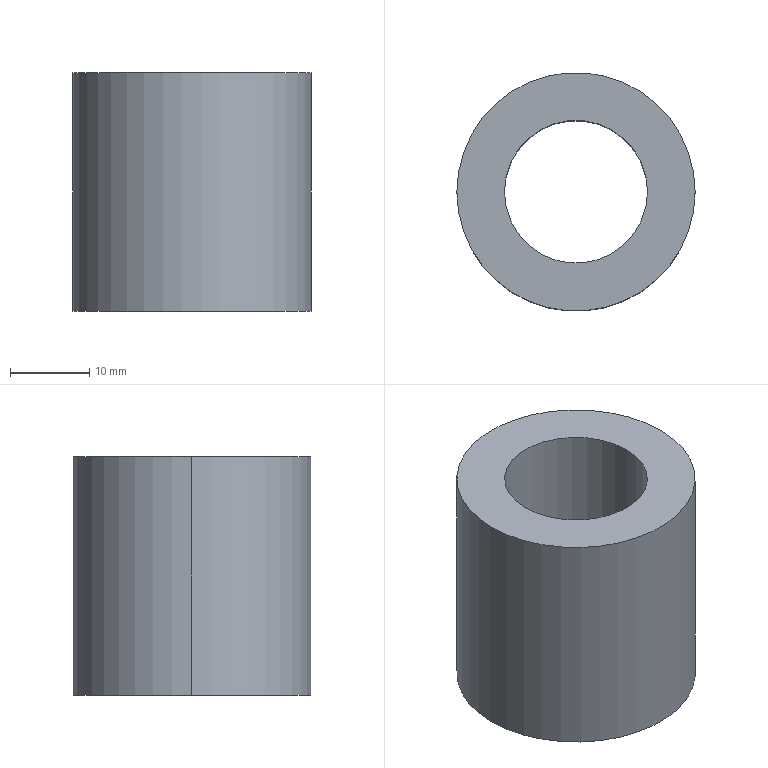Part | STEP file | BCC3 H12_14 | 1 solid | 6 faces | box 30 x 30 x 30 mm | volume 13572 mm3 | cylinder 4 | plane 2 | commonest cylinder face diameters 18 x2 30 x2
STEP:
#1=CARTESIAN_POINT('',(0.,0.,0.));
#2=DIRECTION('',(0.,0.,1.));
#3=DIRECTION('',(1.,0.,0.));
#4=AXIS2_PLACEMENT_3D('',#1,#2,#3);
#5=CARTESIAN_POINT('',(-9.,0.,30.));
#6=VERTEX_POINT('',#5);
#7=CARTESIAN_POINT('',(-9.,0.,0.));
#8=VERTEX_POINT('',#7);
#9=CARTESIAN_POINT('',(-9.,0.,30.));
#10=DIRECTION('',(0.,0.,-1.));
#11=VECTOR('',#10,1.);
#12=LINE('',#9,#11);
#13=CARTESIAN_POINT('',(0.,0.,30.));
#14=DIRECTION('',(0.,0.,-1.));
#15=DIRECTION('',(-1.,0.,0.));
#16=AXIS2_PLACEMENT_3D('',#13,#14,#15);
#17=CYLINDRICAL_SURFACE('',#16,9.);
#18=CARTESIAN_POINT('',(6.283,0.));
#19=DIRECTION('',(0.,1.));
#20=VECTOR('',#19,1.);
#21=LINE('',#18,#20);
#22=(GEOMETRIC_REPRESENTATION_CONTEXT(2)PARAMETRIC_REPRESENTATION_CONTEXT()REPRESENTATION_CONTEXT('',''));
#23=DEFINITIONAL_REPRESENTATION('',(#21),#22);
#24=PCURVE('',#17,#23);
#25=CARTESIAN_POINT('',(0.,0.,30.));
#26=DIRECTION('',(0.,0.,-1.));
#27=DIRECTION('',(-1.,0.,0.));
#28=AXIS2_PLACEMENT_3D('',#25,#26,#27);
#29=CYLINDRICAL_SURFACE('',#28,9.);
#30=CARTESIAN_POINT('',(0.,0.));
#31=DIRECTION('',(0.,1.));
#32=VECTOR('',#31,1.);
#33=LINE('',#30,#32);
#34=(GEOMETRIC_REPRESENTATION_CONTEXT(2)PARAMETRIC_REPRESENTATION_CONTEXT()REPRESENTATION_CONTEXT('',''));
#35=DEFINITIONAL_REPRESENTATION('',(#33),#34);
#36=PCURVE('',#29,#35);
#37=SURFACE_CURVE('',#12,(#24,#36),.PCURVE_S1.);
#38=EDGE_CURVE('',#6,#8,#37,.T.);
#39=ORIENTED_EDGE('',*,*,#38,.T.);
#40=CARTESIAN_POINT('',(9.,0.,0.));
#41=VERTEX_POINT('',#40);
#42=CARTESIAN_POINT('',(0.,0.,0.));
#43=DIRECTION('',(0.,0.,1.));
#44=DIRECTION('',(1.,0.,0.));
#45=AXIS2_PLACEMENT_3D('',#42,#43,#44);
#46=CIRCLE('',#45,9.);
#47=CARTESIAN_POINT('',(9.425,30.));
#48=DIRECTION('',(-1.,0.));
#49=VECTOR('',#48,1.);
#50=LINE('',#47,#49);
#51=(GEOMETRIC_REPRESENTATION_CONTEXT(2)PARAMETRIC_REPRESENTATION_CONTEXT()REPRESENTATION_CONTEXT('',''));
#52=DEFINITIONAL_REPRESENTATION('',(#50),#51);
#53=PCURVE('',#17,#52);
#54=CARTESIAN_POINT('',(0.,0.,0.));
#55=DIRECTION('',(0.,0.,1.));
#56=DIRECTION('',(1.,0.,0.));
#57=AXIS2_PLACEMENT_3D('',#54,#55,#56);
#58=PLANE('',#57);
#59=CARTESIAN_POINT('',(0.,0.));
#60=DIRECTION('',(1.,0.));
#61=AXIS2_PLACEMENT_2D('',#59,#60);
#62=CIRCLE('',#61,9.);
#63=(GEOMETRIC_REPRESENTATION_CONTEXT(2)PARAMETRIC_REPRESENTATION_CONTEXT()REPRESENTATION_CONTEXT('',''));
#64=DEFINITIONAL_REPRESENTATION('',(#62),#63);
#65=PCURVE('',#58,#64);
#66=SURFACE_CURVE('',#46,(#53,#65),.PCURVE_S1.);
#67=EDGE_CURVE('',#8,#41,#66,.T.);
#68=ORIENTED_EDGE('',*,*,#67,.T.);
#69=CARTESIAN_POINT('',(9.,0.,30.));
#70=VERTEX_POINT('',#69);
#71=CARTESIAN_POINT('',(9.,0.,30.));
#72=DIRECTION('',(0.,0.,-1.));
#73=VECTOR('',#72,1.);
#74=LINE('',#71,#73);
#75=CARTESIAN_POINT('',(3.142,0.));
#76=DIRECTION('',(0.,1.));
#77=VECTOR('',#76,1.);
#78=LINE('',#75,#77);
#79=(GEOMETRIC_REPRESENTATION_CONTEXT(2)PARAMETRIC_REPRESENTATION_CONTEXT()REPRESENTATION_CONTEXT('',''));
#80=DEFINITIONAL_REPRESENTATION('',(#78),#79);
#81=PCURVE('',#17,#80);
#82=CARTESIAN_POINT('',(3.142,0.));
#83=DIRECTION('',(0.,1.));
#84=VECTOR('',#83,1.);
#85=LINE('',#82,#84);
#86=(GEOMETRIC_REPRESENTATION_CONTEXT(2)PARAMETRIC_REPRESENTATION_CONTEXT()REPRESENTATION_CONTEXT('',''));
#87=DEFINITIONAL_REPRESENTATION('',(#85),#86);
#88=PCURVE('',#29,#87);
#89=SURFACE_CURVE('',#74,(#81,#88),.PCURVE_S1.);
#90=EDGE_CURVE('',#70,#41,#89,.T.);
#91=ORIENTED_EDGE('',*,*,#90,.F.);
#92=CARTESIAN_POINT('',(0.,0.,30.));
#93=DIRECTION('',(0.,0.,1.));
#94=DIRECTION('',(1.,0.,0.));
#95=AXIS2_PLACEMENT_3D('',#92,#93,#94);
#96=CIRCLE('',#95,9.);
#97=CARTESIAN_POINT('',(9.425,0.));
#98=DIRECTION('',(-1.,0.));
#99=VECTOR('',#98,1.);
#100=LINE('',#97,#99);
#101=(GEOMETRIC_REPRESENTATION_CONTEXT(2)PARAMETRIC_REPRESENTATION_CONTEXT()REPRESENTATION_CONTEXT('',''));
#102=DEFINITIONAL_REPRESENTATION('',(#100),#101);
#103=PCURVE('',#17,#102);
#104=CARTESIAN_POINT('',(0.,0.,30.));
#105=DIRECTION('',(0.,0.,1.));
#106=DIRECTION('',(1.,0.,0.));
#107=AXIS2_PLACEMENT_3D('',#104,#105,#106);
#108=PLANE('',#107);
#109=CARTESIAN_POINT('',(0.,0.));
#110=DIRECTION('',(1.,0.));
#111=AXIS2_PLACEMENT_2D('',#109,#110);
#112=CIRCLE('',#111,9.);
#113=(GEOMETRIC_REPRESENTATION_CONTEXT(2)PARAMETRIC_REPRESENTATION_CONTEXT()REPRESENTATION_CONTEXT('',''));
#114=DEFINITIONAL_REPRESENTATION('',(#112),#113);
#115=PCURVE('',#108,#114);
#116=SURFACE_CURVE('',#96,(#103,#115),.PCURVE_S1.);
#117=EDGE_CURVE('',#6,#70,#116,.T.);
#118=ORIENTED_EDGE('',*,*,#117,.F.);
#119=EDGE_LOOP('',(#39,#68,#91,#118));
#120=FACE_BOUND('',#119,.F.);
#121=ADVANCED_FACE('',(#120),#17,.F.);
#122=CARTESIAN_POINT('',(15.,0.,30.));
#123=VERTEX_POINT('',#122);
#124=CARTESIAN_POINT('',(-15.,0.,30.));
#125=VERTEX_POINT('',#124);
#126=CARTESIAN_POINT('',(0.,0.,30.));
#127=DIRECTION('',(0.,0.,1.));
#128=DIRECTION('',(1.,0.,0.));
#129=AXIS2_PLACEMENT_3D('',#126,#127,#128);
#130=CIRCLE('',#129,15.);
#131=CARTESIAN_POINT('',(0.,0.,30.));
#132=DIRECTION('',(0.,0.,-1.));
#133=DIRECTION('',(-1.,0.,0.));
#134=AXIS2_PLACEMENT_3D('',#131,#132,#133);
#135=CYLINDRICAL_SURFACE('',#134,15.);
#136=CARTESIAN_POINT('',(3.142,0.));
#137=DIRECTION('',(-1.,0.));
#138=VECTOR('',#137,1.);
#139=LINE('',#136,#138);
#140=(GEOMETRIC_REPRESENTATION_CONTEXT(2)PARAMETRIC_REPRESENTATION_CONTEXT()REPRESENTATION_CONTEXT('',''));
#141=DEFINITIONAL_REPRESENTATION('',(#139),#140);
#142=PCURVE('',#135,#141);
#143=CARTESIAN_POINT('',(0.,0.));
#144=DIRECTION('',(1.,0.));
#145=AXIS2_PLACEMENT_2D('',#143,#144);
#146=CIRCLE('',#145,15.);
#147=(GEOMETRIC_REPRESENTATION_CONTEXT(2)PARAMETRIC_REPRESENTATION_CONTEXT()REPRESENTATION_CONTEXT('',''));
#148=DEFINITIONAL_REPRESENTATION('',(#146),#147);
#149=PCURVE('',#108,#148);
#150=SURFACE_CURVE('',#130,(#142,#149),.PCURVE_S1.);
#151=EDGE_CURVE('',#123,#125,#150,.T.);
#152=ORIENTED_EDGE('',*,*,#151,.F.);
#153=CARTESIAN_POINT('',(15.,0.,0.));
#154=VERTEX_POINT('',#153);
#155=CARTESIAN_POINT('',(15.,0.,30.));
#156=DIRECTION('',(0.,0.,-1.));
#157=VECTOR('',#156,1.);
#158=LINE('',#155,#157);
#159=CARTESIAN_POINT('',(3.142,0.));
#160=DIRECTION('',(0.,1.));
#161=VECTOR('',#160,1.);
#162=LINE('',#159,#161);
#163=(GEOMETRIC_REPRESENTATION_CONTEXT(2)PARAMETRIC_REPRESENTATION_CONTEXT()REPRESENTATION_CONTEXT('',''));
#164=DEFINITIONAL_REPRESENTATION('',(#162),#163);
#165=PCURVE('',#135,#164);
#166=CARTESIAN_POINT('',(0.,0.,30.));
#167=DIRECTION('',(0.,0.,-1.));
#168=DIRECTION('',(-1.,0.,0.));
#169=AXIS2_PLACEMENT_3D('',#166,#167,#168);
#170=CYLINDRICAL_SURFACE('',#169,15.);
#171=CARTESIAN_POINT('',(3.142,0.));
#172=DIRECTION('',(0.,1.));
#173=VECTOR('',#172,1.);
#174=LINE('',#171,#173);
#175=(GEOMETRIC_REPRESENTATION_CONTEXT(2)PARAMETRIC_REPRESENTATION_CONTEXT()REPRESENTATION_CONTEXT('',''));
#176=DEFINITIONAL_REPRESENTATION('',(#174),#175);
#177=PCURVE('',#170,#176);
#178=SURFACE_CURVE('',#158,(#165,#177),.PCURVE_S1.);
#179=EDGE_CURVE('',#123,#154,#178,.T.);
#180=ORIENTED_EDGE('',*,*,#179,.T.);
#181=CARTESIAN_POINT('',(-15.,0.,0.));
#182=VERTEX_POINT('',#181);
#183=CARTESIAN_POINT('',(0.,0.,0.));
#184=DIRECTION('',(0.,0.,1.));
#185=DIRECTION('',(1.,0.,0.));
#186=AXIS2_PLACEMENT_3D('',#183,#184,#185);
#187=CIRCLE('',#186,15.);
#188=CARTESIAN_POINT('',(3.142,30.));
#189=DIRECTION('',(-1.,0.));
#190=VECTOR('',#189,1.);
#191=LINE('',#188,#190);
#192=(GEOMETRIC_REPRESENTATION_CONTEXT(2)PARAMETRIC_REPRESENTATION_CONTEXT()REPRESENTATION_CONTEXT('',''));
#193=DEFINITIONAL_REPRESENTATION('',(#191),#192);
#194=PCURVE('',#135,#193);
#195=CARTESIAN_POINT('',(0.,0.));
#196=DIRECTION('',(1.,0.));
#197=AXIS2_PLACEMENT_2D('',#195,#196);
#198=CIRCLE('',#197,15.);
#199=(GEOMETRIC_REPRESENTATION_CONTEXT(2)PARAMETRIC_REPRESENTATION_CONTEXT()REPRESENTATION_CONTEXT('',''));
#200=DEFINITIONAL_REPRESENTATION('',(#198),#199);
#201=PCURVE('',#58,#200);
#202=SURFACE_CURVE('',#187,(#194,#201),.PCURVE_S1.);
#203=EDGE_CURVE('',#154,#182,#202,.T.);
#204=ORIENTED_EDGE('',*,*,#203,.T.);
#205=CARTESIAN_POINT('',(-15.,0.,30.));
#206=DIRECTION('',(0.,0.,-1.));
#207=VECTOR('',#206,1.);
#208=LINE('',#205,#207);
#209=CARTESIAN_POINT('',(0.,0.));
#210=DIRECTION('',(0.,1.));
#211=VECTOR('',#210,1.);
#212=LINE('',#209,#211);
#213=(GEOMETRIC_REPRESENTATION_CONTEXT(2)PARAMETRIC_REPRESENTATION_CONTEXT()REPRESENTATION_CONTEXT('',''));
#214=DEFINITIONAL_REPRESENTATION('',(#212),#213);
#215=PCURVE('',#135,#214);
#216=CARTESIAN_POINT('',(6.283,0.));
#217=DIRECTION('',(0.,1.));
#218=VECTOR('',#217,1.);
#219=LINE('',#216,#218);
#220=(GEOMETRIC_REPRESENTATION_CONTEXT(2)PARAMETRIC_REPRESENTATION_CONTEXT()REPRESENTATION_CONTEXT('',''));
#221=DEFINITIONAL_REPRESENTATION('',(#219),#220);
#222=PCURVE('',#170,#221);
#223=SURFACE_CURVE('',#208,(#215,#222),.PCURVE_S1.);
#224=EDGE_CURVE('',#125,#182,#223,.T.);
#225=ORIENTED_EDGE('',*,*,#224,.F.);
#226=EDGE_LOOP('',(#152,#180,#204,#225));
#227=FACE_BOUND('',#226,.T.);
#228=ADVANCED_FACE('',(#227),#135,.T.);
#229=CARTESIAN_POINT('',(0.,0.,30.));
#230=DIRECTION('',(0.,0.,1.));
#231=DIRECTION('',(1.,0.,0.));
#232=AXIS2_PLACEMENT_3D('',#229,#230,#231);
#233=CIRCLE('',#232,15.);
#234=CARTESIAN_POINT('',(0.,0.));
#235=DIRECTION('',(1.,0.));
#236=AXIS2_PLACEMENT_2D('',#234,#235);
#237=CIRCLE('',#236,15.);
#238=(GEOMETRIC_REPRESENTATION_CONTEXT(2)PARAMETRIC_REPRESENTATION_CONTEXT()REPRESENTATION_CONTEXT('',''));
#239=DEFINITIONAL_REPRESENTATION('',(#237),#238);
#240=PCURVE('',#108,#239);
#241=CARTESIAN_POINT('',(9.425,0.));
#242=DIRECTION('',(-1.,0.));
#243=VECTOR('',#242,1.);
#244=LINE('',#241,#243);
#245=(GEOMETRIC_REPRESENTATION_CONTEXT(2)PARAMETRIC_REPRESENTATION_CONTEXT()REPRESENTATION_CONTEXT('',''));
#246=DEFINITIONAL_REPRESENTATION('',(#244),#245);
#247=PCURVE('',#170,#246);
#248=SURFACE_CURVE('',#233,(#240,#247),.PCURVE_S1.);
#249=EDGE_CURVE('',#125,#123,#248,.T.);
#250=ORIENTED_EDGE('',*,*,#249,.T.);
#251=ORIENTED_EDGE('',*,*,#151,.T.);
#252=EDGE_LOOP('',(#250,#251));
#253=FACE_BOUND('',#252,.T.);
#254=ORIENTED_EDGE('',*,*,#117,.F.);
#255=CARTESIAN_POINT('',(0.,0.,30.));
#256=DIRECTION('',(0.,0.,1.));
#257=DIRECTION('',(1.,0.,0.));
#258=AXIS2_PLACEMENT_3D('',#255,#256,#257);
#259=CIRCLE('',#258,9.);
#260=CARTESIAN_POINT('',(0.,0.));
#261=DIRECTION('',(1.,0.));
#262=AXIS2_PLACEMENT_2D('',#260,#261);
#263=CIRCLE('',#262,9.);
#264=(GEOMETRIC_REPRESENTATION_CONTEXT(2)PARAMETRIC_REPRESENTATION_CONTEXT()REPRESENTATION_CONTEXT('',''));
#265=DEFINITIONAL_REPRESENTATION('',(#263),#264);
#266=PCURVE('',#108,#265);
#267=CARTESIAN_POINT('',(3.142,0.));
#268=DIRECTION('',(-1.,0.));
#269=VECTOR('',#268,1.);
#270=LINE('',#267,#269);
#271=(GEOMETRIC_REPRESENTATION_CONTEXT(2)PARAMETRIC_REPRESENTATION_CONTEXT()REPRESENTATION_CONTEXT('',''));
#272=DEFINITIONAL_REPRESENTATION('',(#270),#271);
#273=PCURVE('',#29,#272);
#274=SURFACE_CURVE('',#259,(#266,#273),.PCURVE_S1.);
#275=EDGE_CURVE('',#70,#6,#274,.T.);
#276=ORIENTED_EDGE('',*,*,#275,.F.);
#277=EDGE_LOOP('',(#254,#276));
#278=FACE_BOUND('',#277,.T.);
#279=ADVANCED_FACE('',(#253,#278),#108,.T.);
#280=CARTESIAN_POINT('',(0.,0.,0.));
#281=DIRECTION('',(0.,0.,1.));
#282=DIRECTION('',(1.,0.,0.));
#283=AXIS2_PLACEMENT_3D('',#280,#281,#282);
#284=CIRCLE('',#283,15.);
#285=CARTESIAN_POINT('',(0.,0.));
#286=DIRECTION('',(1.,0.));
#287=AXIS2_PLACEMENT_2D('',#285,#286);
#288=CIRCLE('',#287,15.);
#289=(GEOMETRIC_REPRESENTATION_CONTEXT(2)PARAMETRIC_REPRESENTATION_CONTEXT()REPRESENTATION_CONTEXT('',''));
#290=DEFINITIONAL_REPRESENTATION('',(#288),#289);
#291=PCURVE('',#58,#290);
#292=CARTESIAN_POINT('',(9.425,30.));
#293=DIRECTION('',(-1.,0.));
#294=VECTOR('',#293,1.);
#295=LINE('',#292,#294);
#296=(GEOMETRIC_REPRESENTATION_CONTEXT(2)PARAMETRIC_REPRESENTATION_CONTEXT()REPRESENTATION_CONTEXT('',''));
#297=DEFINITIONAL_REPRESENTATION('',(#295),#296);
#298=PCURVE('',#170,#297);
#299=SURFACE_CURVE('',#284,(#291,#298),.PCURVE_S1.);
#300=EDGE_CURVE('',#182,#154,#299,.T.);
#301=ORIENTED_EDGE('',*,*,#300,.F.);
#302=ORIENTED_EDGE('',*,*,#203,.F.);
#303=EDGE_LOOP('',(#301,#302));
#304=FACE_BOUND('',#303,.T.);
#305=ORIENTED_EDGE('',*,*,#67,.T.);
#306=CARTESIAN_POINT('',(0.,0.,0.));
#307=DIRECTION('',(0.,0.,1.));
#308=DIRECTION('',(1.,0.,0.));
#309=AXIS2_PLACEMENT_3D('',#306,#307,#308);
#310=CIRCLE('',#309,9.);
#311=CARTESIAN_POINT('',(0.,0.));
#312=DIRECTION('',(1.,0.));
#313=AXIS2_PLACEMENT_2D('',#311,#312);
#314=CIRCLE('',#313,9.);
#315=(GEOMETRIC_REPRESENTATION_CONTEXT(2)PARAMETRIC_REPRESENTATION_CONTEXT()REPRESENTATION_CONTEXT('',''));
#316=DEFINITIONAL_REPRESENTATION('',(#314),#315);
#317=PCURVE('',#58,#316);
#318=CARTESIAN_POINT('',(3.142,30.));
#319=DIRECTION('',(-1.,0.));
#320=VECTOR('',#319,1.);
#321=LINE('',#318,#320);
#322=(GEOMETRIC_REPRESENTATION_CONTEXT(2)PARAMETRIC_REPRESENTATION_CONTEXT()REPRESENTATION_CONTEXT('',''));
#323=DEFINITIONAL_REPRESENTATION('',(#321),#322);
#324=PCURVE('',#29,#323);
#325=SURFACE_CURVE('',#310,(#317,#324),.PCURVE_S1.);
#326=EDGE_CURVE('',#41,#8,#325,.T.);
#327=ORIENTED_EDGE('',*,*,#326,.T.);
#328=EDGE_LOOP('',(#305,#327));
#329=FACE_BOUND('',#328,.T.);
#330=ADVANCED_FACE('',(#304,#329),#58,.F.);
#331=ORIENTED_EDGE('',*,*,#179,.F.);
#332=ORIENTED_EDGE('',*,*,#249,.F.);
#333=ORIENTED_EDGE('',*,*,#224,.T.);
#334=ORIENTED_EDGE('',*,*,#300,.T.);
#335=EDGE_LOOP('',(#331,#332,#333,#334));
#336=FACE_BOUND('',#335,.T.);
#337=ADVANCED_FACE('',(#336),#170,.T.);
#338=ORIENTED_EDGE('',*,*,#326,.T.);
#339=ORIENTED_EDGE('',*,*,#38,.F.);
#340=ORIENTED_EDGE('',*,*,#275,.F.);
#341=ORIENTED_EDGE('',*,*,#90,.T.);
#342=EDGE_LOOP('',(#338,#339,#340,#341));
#343=FACE_BOUND('',#342,.F.);
#344=ADVANCED_FACE('',(#343),#29,.F.);
#345=CLOSED_SHELL('',(#121,#228,#279,#330,#337,#344));
#346=MANIFOLD_SOLID_BREP('',#345);
#347=(LENGTH_UNIT()NAMED_UNIT(*)SI_UNIT(.MILLI.,.METRE.));
#348=UNCERTAINTY_MEASURE_WITH_UNIT(LENGTH_MEASURE(0.0000001),#347,'','');
#349=(NAMED_UNIT(*)PLANE_ANGLE_UNIT()SI_UNIT($,.RADIAN.));
#350=(NAMED_UNIT(*)SI_UNIT($,.STERADIAN.)SOLID_ANGLE_UNIT());
#351=(GEOMETRIC_REPRESENTATION_CONTEXT(3)GLOBAL_UNCERTAINTY_ASSIGNED_CONTEXT((#348))GLOBAL_UNIT_ASSIGNED_CONTEXT((#347,#349,#350))REPRESENTATION_CONTEXT('',''));
#352=ADVANCED_BREP_SHAPE_REPRESENTATION('',(#4,#346),#351);